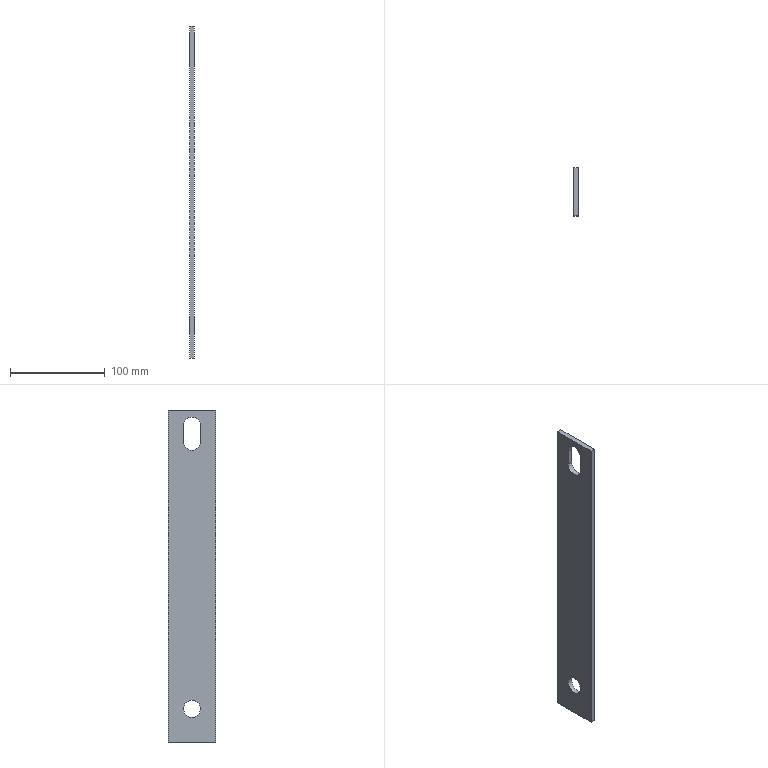Part | NX | features solid 2 | 1 solid | 11 faces | box 5 x 50 x 350 mm | volume 83425 mm3 | plane 8 | cylinder 3 | commonest cylinder face diameters 18 x3
STEP:
#1=CARTESIAN_POINT('',(1485.,754.,143.5));
#2=VERTEX_POINT('',#1);
#3=CARTESIAN_POINT('',(1490.,754.,143.5));
#4=VERTEX_POINT('',#3);
#5=CARTESIAN_POINT('',(1487.5,754.,143.5));
#6=DIRECTION('',(1.,0.,0.));
#7=VECTOR('',#6,1000.);
#8=LINE('',#5,#7);
#9=EDGE_CURVE('',#2,#4,#8,.T.);
#10=ORIENTED_EDGE('',*,*,#9,.T.);
#11=CARTESIAN_POINT('',(1490.,736.,143.5));
#12=VERTEX_POINT('',#11);
#13=CARTESIAN_POINT('',(1490.,745.,143.5));
#14=DIRECTION('',(-1.,0.,0.));
#15=DIRECTION('',(0.,0.,-1.));
#16=AXIS2_PLACEMENT_3D('',#13,#14,#15);
#17=CIRCLE('',#16,9.);
#18=EDGE_CURVE('',#12,#4,#17,.T.);
#19=ORIENTED_EDGE('',*,*,#18,.F.);
#20=CARTESIAN_POINT('',(1485.,736.,143.5));
#21=VERTEX_POINT('',#20);
#22=CARTESIAN_POINT('',(1487.5,736.,143.5));
#23=DIRECTION('',(-1.,0.,0.));
#24=VECTOR('',#23,1000.);
#25=LINE('',#22,#24);
#26=EDGE_CURVE('',#12,#21,#25,.T.);
#27=ORIENTED_EDGE('',*,*,#26,.T.);
#28=CARTESIAN_POINT('',(1485.,745.,143.5));
#29=DIRECTION('',(1.,0.,0.));
#30=DIRECTION('',(0.,0.,1.));
#31=AXIS2_PLACEMENT_3D('',#28,#29,#30);
#32=CIRCLE('',#31,9.);
#33=EDGE_CURVE('',#2,#21,#32,.T.);
#34=ORIENTED_EDGE('',*,*,#33,.F.);
#35=EDGE_LOOP('',(#10,#19,#27,#34));
#36=FACE_BOUND('',#35,.T.);
#37=CARTESIAN_POINT('',(1485.,745.,143.5));
#38=DIRECTION('',(1.,0.,0.));
#39=DIRECTION('',(0.,0.,1.));
#40=AXIS2_PLACEMENT_3D('',#37,#38,#39);
#41=CYLINDRICAL_SURFACE('',#40,9.);
#42=ADVANCED_FACE('',(#36),#41,.F.);
#43=CARTESIAN_POINT('',(1485.,770.,160.));
#44=VERTEX_POINT('',#43);
#45=CARTESIAN_POINT('',(1490.,770.,160.));
#46=VERTEX_POINT('',#45);
#47=CARTESIAN_POINT('',(1487.5,770.,160.));
#48=DIRECTION('',(1.,0.,0.));
#49=VECTOR('',#48,1000.);
#50=LINE('',#47,#49);
#51=EDGE_CURVE('',#44,#46,#50,.T.);
#52=ORIENTED_EDGE('',*,*,#51,.F.);
#53=CARTESIAN_POINT('',(1485.,720.,160.));
#54=VERTEX_POINT('',#53);
#55=CARTESIAN_POINT('',(1485.,745.,160.));
#56=DIRECTION('',(0.,1.,0.));
#57=VECTOR('',#56,1000.);
#58=LINE('',#55,#57);
#59=EDGE_CURVE('',#54,#44,#58,.T.);
#60=ORIENTED_EDGE('',*,*,#59,.F.);
#61=CARTESIAN_POINT('',(1490.,720.,160.));
#62=VERTEX_POINT('',#61);
#63=CARTESIAN_POINT('',(1487.5,720.,160.));
#64=DIRECTION('',(-1.,0.,0.));
#65=VECTOR('',#64,1000.);
#66=LINE('',#63,#65);
#67=EDGE_CURVE('',#62,#54,#66,.T.);
#68=ORIENTED_EDGE('',*,*,#67,.F.);
#69=CARTESIAN_POINT('',(1490.,745.,160.));
#70=DIRECTION('',(0.,-1.,0.));
#71=VECTOR('',#70,1000.);
#72=LINE('',#69,#71);
#73=EDGE_CURVE('',#46,#62,#72,.T.);
#74=ORIENTED_EDGE('',*,*,#73,.F.);
#75=EDGE_LOOP('',(#52,#60,#68,#74));
#76=FACE_BOUND('',#75,.T.);
#77=CARTESIAN_POINT('',(1477.5,745.,160.));
#78=DIRECTION('',(0.,0.,1.));
#79=DIRECTION('',(-1.,0.,0.));
#80=AXIS2_PLACEMENT_3D('',#77,#78,#79);
#81=PLANE('',#80);
#82=ADVANCED_FACE('',(#76),#81,.T.);
#83=CARTESIAN_POINT('',(1490.,770.,-190.));
#84=VERTEX_POINT('',#83);
#85=CARTESIAN_POINT('',(1490.,770.,-105.));
#86=DIRECTION('',(0.,0.,1.));
#87=VECTOR('',#86,1000.);
#88=LINE('',#85,#87);
#89=EDGE_CURVE('',#84,#46,#88,.T.);
#90=ORIENTED_EDGE('',*,*,#89,.F.);
#91=CARTESIAN_POINT('',(1485.,770.,-190.));
#92=VERTEX_POINT('',#91);
#93=CARTESIAN_POINT('',(1487.5,770.,-190.));
#94=DIRECTION('',(-1.,0.,0.));
#95=VECTOR('',#94,1000.);
#96=LINE('',#93,#95);
#97=EDGE_CURVE('',#84,#92,#96,.T.);
#98=ORIENTED_EDGE('',*,*,#97,.T.);
#99=CARTESIAN_POINT('',(1485.,770.,-105.));
#100=DIRECTION('',(0.,0.,1.));
#101=VECTOR('',#100,1000.);
#102=LINE('',#99,#101);
#103=EDGE_CURVE('',#92,#44,#102,.T.);
#104=ORIENTED_EDGE('',*,*,#103,.T.);
#105=ORIENTED_EDGE('',*,*,#51,.T.);
#106=EDGE_LOOP('',(#90,#98,#104,#105));
#107=FACE_BOUND('',#106,.T.);
#108=CARTESIAN_POINT('',(1487.5,770.,-105.));
#109=DIRECTION('',(0.,1.,0.));
#110=DIRECTION('',(0.,0.,-1.));
#111=AXIS2_PLACEMENT_3D('',#108,#109,#110);
#112=PLANE('',#111);
#113=ADVANCED_FACE('',(#107),#112,.T.);
#114=CARTESIAN_POINT('',(1490.,720.,-190.));
#115=VERTEX_POINT('',#114);
#116=CARTESIAN_POINT('',(1490.,720.,-105.));
#117=DIRECTION('',(0.,0.,1.));
#118=VECTOR('',#117,1000.);
#119=LINE('',#116,#118);
#120=EDGE_CURVE('',#115,#62,#119,.T.);
#121=ORIENTED_EDGE('',*,*,#120,.F.);
#122=CARTESIAN_POINT('',(1490.,745.,-190.));
#123=DIRECTION('',(0.,1.,0.));
#124=VECTOR('',#123,1000.);
#125=LINE('',#122,#124);
#126=EDGE_CURVE('',#115,#84,#125,.T.);
#127=ORIENTED_EDGE('',*,*,#126,.T.);
#128=ORIENTED_EDGE('',*,*,#89,.T.);
#129=ORIENTED_EDGE('',*,*,#73,.T.);
#130=EDGE_LOOP('',(#121,#127,#128,#129));
#131=FACE_BOUND('',#130,.T.);
#132=CARTESIAN_POINT('',(1490.,754.,126.5));
#133=VERTEX_POINT('',#132);
#134=CARTESIAN_POINT('',(1490.,754.,126.5));
#135=DIRECTION('',(0.,0.,1.));
#136=VECTOR('',#135,1000.);
#137=LINE('',#134,#136);
#138=EDGE_CURVE('',#133,#4,#137,.T.);
#139=ORIENTED_EDGE('',*,*,#138,.F.);
#140=CARTESIAN_POINT('',(1490.,736.,126.5));
#141=VERTEX_POINT('',#140);
#142=CARTESIAN_POINT('',(1490.,745.,126.5));
#143=DIRECTION('',(-1.,0.,0.));
#144=DIRECTION('',(0.,0.,-1.));
#145=AXIS2_PLACEMENT_3D('',#142,#143,#144);
#146=CIRCLE('',#145,9.);
#147=EDGE_CURVE('',#133,#141,#146,.T.);
#148=ORIENTED_EDGE('',*,*,#147,.T.);
#149=CARTESIAN_POINT('',(1490.,736.,126.5));
#150=DIRECTION('',(0.,0.,1.));
#151=VECTOR('',#150,1000.);
#152=LINE('',#149,#151);
#153=EDGE_CURVE('',#141,#12,#152,.T.);
#154=ORIENTED_EDGE('',*,*,#153,.T.);
#155=ORIENTED_EDGE('',*,*,#18,.T.);
#156=EDGE_LOOP('',(#139,#148,#154,#155));
#157=FACE_BOUND('',#156,.T.);
#158=CARTESIAN_POINT('',(1490.,745.,-164.));
#159=VERTEX_POINT('',#158);
#160=CARTESIAN_POINT('',(1490.,745.,-155.));
#161=DIRECTION('',(-1.,0.,0.));
#162=DIRECTION('',(0.,0.,-1.));
#163=AXIS2_PLACEMENT_3D('',#160,#161,#162);
#164=CIRCLE('',#163,9.);
#165=EDGE_CURVE('',#159,#159,#164,.T.);
#166=ORIENTED_EDGE('',*,*,#165,.T.);
#167=EDGE_LOOP('',(#166));
#168=FACE_BOUND('',#167,.T.);
#169=CARTESIAN_POINT('',(1490.,745.,-105.));
#170=DIRECTION('',(1.,0.,0.));
#171=DIRECTION('',(0.,0.,1.));
#172=AXIS2_PLACEMENT_3D('',#169,#170,#171);
#173=PLANE('',#172);
#174=ADVANCED_FACE('',(#131,#157,#168),#173,.T.);
#175=CARTESIAN_POINT('',(1485.,720.,-190.));
#176=VERTEX_POINT('',#175);
#177=CARTESIAN_POINT('',(1485.,720.,-105.));
#178=DIRECTION('',(0.,0.,1.));
#179=VECTOR('',#178,1000.);
#180=LINE('',#177,#179);
#181=EDGE_CURVE('',#176,#54,#180,.T.);
#182=ORIENTED_EDGE('',*,*,#181,.F.);
#183=CARTESIAN_POINT('',(1487.5,720.,-190.));
#184=DIRECTION('',(1.,0.,0.));
#185=VECTOR('',#184,1000.);
#186=LINE('',#183,#185);
#187=EDGE_CURVE('',#176,#115,#186,.T.);
#188=ORIENTED_EDGE('',*,*,#187,.T.);
#189=ORIENTED_EDGE('',*,*,#120,.T.);
#190=ORIENTED_EDGE('',*,*,#67,.T.);
#191=EDGE_LOOP('',(#182,#188,#189,#190));
#192=FACE_BOUND('',#191,.T.);
#193=CARTESIAN_POINT('',(1487.5,720.,-105.));
#194=DIRECTION('',(0.,-1.,0.));
#195=DIRECTION('',(0.,0.,1.));
#196=AXIS2_PLACEMENT_3D('',#193,#194,#195);
#197=PLANE('',#196);
#198=ADVANCED_FACE('',(#192),#197,.T.);
#199=ORIENTED_EDGE('',*,*,#103,.F.);
#200=CARTESIAN_POINT('',(1485.,745.,-190.));
#201=DIRECTION('',(0.,-1.,0.));
#202=VECTOR('',#201,1000.);
#203=LINE('',#200,#202);
#204=EDGE_CURVE('',#92,#176,#203,.T.);
#205=ORIENTED_EDGE('',*,*,#204,.T.);
#206=ORIENTED_EDGE('',*,*,#181,.T.);
#207=ORIENTED_EDGE('',*,*,#59,.T.);
#208=EDGE_LOOP('',(#199,#205,#206,#207));
#209=FACE_BOUND('',#208,.T.);
#210=CARTESIAN_POINT('',(1485.,754.,126.5));
#211=VERTEX_POINT('',#210);
#212=CARTESIAN_POINT('',(1485.,754.,126.5));
#213=DIRECTION('',(0.,0.,1.));
#214=VECTOR('',#213,1000.);
#215=LINE('',#212,#214);
#216=EDGE_CURVE('',#211,#2,#215,.T.);
#217=ORIENTED_EDGE('',*,*,#216,.T.);
#218=ORIENTED_EDGE('',*,*,#33,.T.);
#219=CARTESIAN_POINT('',(1485.,736.,126.5));
#220=VERTEX_POINT('',#219);
#221=CARTESIAN_POINT('',(1485.,736.,126.5));
#222=DIRECTION('',(0.,0.,1.));
#223=VECTOR('',#222,1000.);
#224=LINE('',#221,#223);
#225=EDGE_CURVE('',#220,#21,#224,.T.);
#226=ORIENTED_EDGE('',*,*,#225,.F.);
#227=CARTESIAN_POINT('',(1485.,745.,126.5));
#228=DIRECTION('',(1.,0.,0.));
#229=DIRECTION('',(0.,0.,1.));
#230=AXIS2_PLACEMENT_3D('',#227,#228,#229);
#231=CIRCLE('',#230,9.);
#232=EDGE_CURVE('',#220,#211,#231,.T.);
#233=ORIENTED_EDGE('',*,*,#232,.T.);
#234=EDGE_LOOP('',(#217,#218,#226,#233));
#235=FACE_BOUND('',#234,.T.);
#236=CARTESIAN_POINT('',(1485.,745.,-146.));
#237=VERTEX_POINT('',#236);
#238=CARTESIAN_POINT('',(1485.,745.,-155.));
#239=DIRECTION('',(1.,0.,0.));
#240=DIRECTION('',(0.,0.,1.));
#241=AXIS2_PLACEMENT_3D('',#238,#239,#240);
#242=CIRCLE('',#241,9.);
#243=EDGE_CURVE('',#237,#237,#242,.T.);
#244=ORIENTED_EDGE('',*,*,#243,.T.);
#245=EDGE_LOOP('',(#244));
#246=FACE_BOUND('',#245,.T.);
#247=CARTESIAN_POINT('',(1485.,745.,-105.));
#248=DIRECTION('',(-1.,0.,0.));
#249=DIRECTION('',(0.,0.,-1.));
#250=AXIS2_PLACEMENT_3D('',#247,#248,#249);
#251=PLANE('',#250);
#252=ADVANCED_FACE('',(#209,#235,#246),#251,.T.);
#253=ORIENTED_EDGE('',*,*,#147,.F.);
#254=CARTESIAN_POINT('',(1487.5,754.,126.5));
#255=DIRECTION('',(-1.,0.,0.));
#256=VECTOR('',#255,1000.);
#257=LINE('',#254,#256);
#258=EDGE_CURVE('',#133,#211,#257,.T.);
#259=ORIENTED_EDGE('',*,*,#258,.T.);
#260=ORIENTED_EDGE('',*,*,#232,.F.);
#261=CARTESIAN_POINT('',(1487.5,736.,126.5));
#262=DIRECTION('',(1.,0.,0.));
#263=VECTOR('',#262,1000.);
#264=LINE('',#261,#263);
#265=EDGE_CURVE('',#220,#141,#264,.T.);
#266=ORIENTED_EDGE('',*,*,#265,.T.);
#267=EDGE_LOOP('',(#253,#259,#260,#266));
#268=FACE_BOUND('',#267,.T.);
#269=CARTESIAN_POINT('',(1485.,745.,126.5));
#270=DIRECTION('',(1.,0.,0.));
#271=DIRECTION('',(0.,0.,1.));
#272=AXIS2_PLACEMENT_3D('',#269,#270,#271);
#273=CYLINDRICAL_SURFACE('',#272,9.);
#274=ADVANCED_FACE('',(#268),#273,.F.);
#275=ORIENTED_EDGE('',*,*,#153,.F.);
#276=ORIENTED_EDGE('',*,*,#265,.F.);
#277=ORIENTED_EDGE('',*,*,#225,.T.);
#278=ORIENTED_EDGE('',*,*,#26,.F.);
#279=EDGE_LOOP('',(#275,#276,#277,#278));
#280=FACE_BOUND('',#279,.T.);
#281=CARTESIAN_POINT('',(1487.5,736.,126.5));
#282=DIRECTION('',(0.,-1.,0.));
#283=DIRECTION('',(0.,0.,1.));
#284=AXIS2_PLACEMENT_3D('',#281,#282,#283);
#285=PLANE('',#284);
#286=ADVANCED_FACE('',(#280),#285,.F.);
#287=ORIENTED_EDGE('',*,*,#216,.F.);
#288=ORIENTED_EDGE('',*,*,#258,.F.);
#289=ORIENTED_EDGE('',*,*,#138,.T.);
#290=ORIENTED_EDGE('',*,*,#9,.F.);
#291=EDGE_LOOP('',(#287,#288,#289,#290));
#292=FACE_BOUND('',#291,.T.);
#293=CARTESIAN_POINT('',(1487.5,754.,126.5));
#294=DIRECTION('',(0.,1.,0.));
#295=DIRECTION('',(0.,0.,-1.));
#296=AXIS2_PLACEMENT_3D('',#293,#294,#295);
#297=PLANE('',#296);
#298=ADVANCED_FACE('',(#292),#297,.F.);
#299=ORIENTED_EDGE('',*,*,#204,.F.);
#300=ORIENTED_EDGE('',*,*,#97,.F.);
#301=ORIENTED_EDGE('',*,*,#126,.F.);
#302=ORIENTED_EDGE('',*,*,#187,.F.);
#303=EDGE_LOOP('',(#299,#300,#301,#302));
#304=FACE_BOUND('',#303,.T.);
#305=CARTESIAN_POINT('',(1477.5,745.,-190.));
#306=DIRECTION('',(0.,0.,-1.));
#307=DIRECTION('',(1.,0.,0.));
#308=AXIS2_PLACEMENT_3D('',#305,#306,#307);
#309=PLANE('',#308);
#310=ADVANCED_FACE('',(#304),#309,.T.);
#311=ORIENTED_EDGE('',*,*,#165,.F.);
#312=EDGE_LOOP('',(#311));
#313=FACE_BOUND('',#312,.T.);
#314=ORIENTED_EDGE('',*,*,#243,.F.);
#315=EDGE_LOOP('',(#314));
#316=FACE_BOUND('',#315,.T.);
#317=CARTESIAN_POINT('',(1485.,745.,-155.));
#318=DIRECTION('',(1.,0.,0.));
#319=DIRECTION('',(0.,0.,1.));
#320=AXIS2_PLACEMENT_3D('',#317,#318,#319);
#321=CYLINDRICAL_SURFACE('',#320,9.);
#322=ADVANCED_FACE('',(#313,#316),#321,.F.);
#323=CLOSED_SHELL('',(#42,#82,#113,#174,#198,#252,#274,#286,#298,#310,#322));
#324=MANIFOLD_SOLID_BREP('',#323);
#325=(LENGTH_UNIT()NAMED_UNIT(*)SI_UNIT(.MILLI.,.METRE.));
#326=UNCERTAINTY_MEASURE_WITH_UNIT(LENGTH_MEASURE(0.00001),#325,'','');
#327=(NAMED_UNIT(*)PLANE_ANGLE_UNIT()SI_UNIT($,.RADIAN.));
#328=(NAMED_UNIT(*)SI_UNIT($,.STERADIAN.)SOLID_ANGLE_UNIT());
#329=(GEOMETRIC_REPRESENTATION_CONTEXT(3)GLOBAL_UNCERTAINTY_ASSIGNED_CONTEXT((#326))GLOBAL_UNIT_ASSIGNED_CONTEXT((#325,#327,#328))REPRESENTATION_CONTEXT('',''));
#330=ADVANCED_BREP_SHAPE_REPRESENTATION('',(#324),#329);